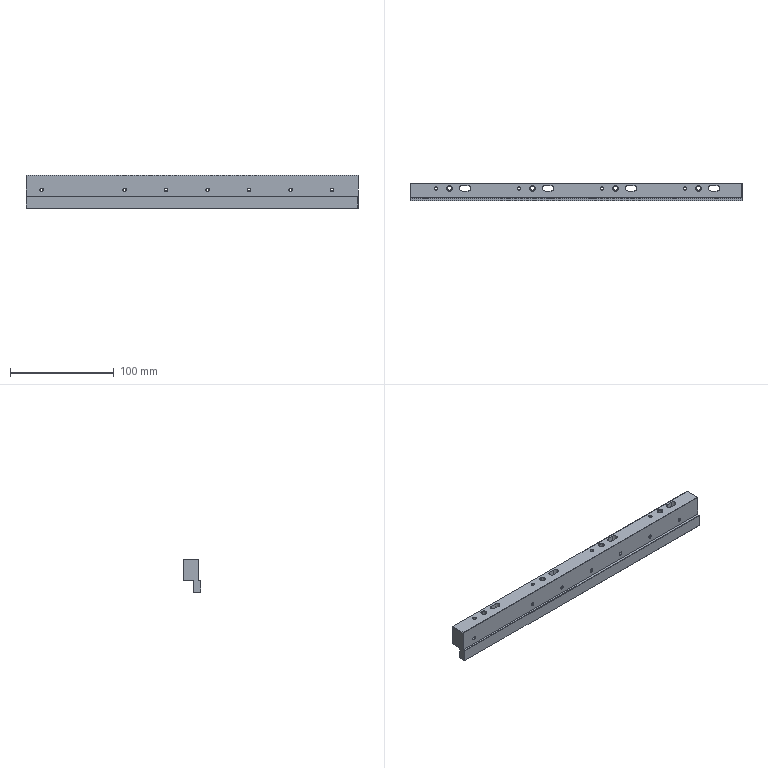Part | NX | 1 solid | 109 faces | box 320 x 17 x 32 mm | volume 113573 mm3 | cylinder 48 | plane 31 | cone 30 | commonest cylinder face diameters 2.5 x28 5.2 x12 4.2 x8